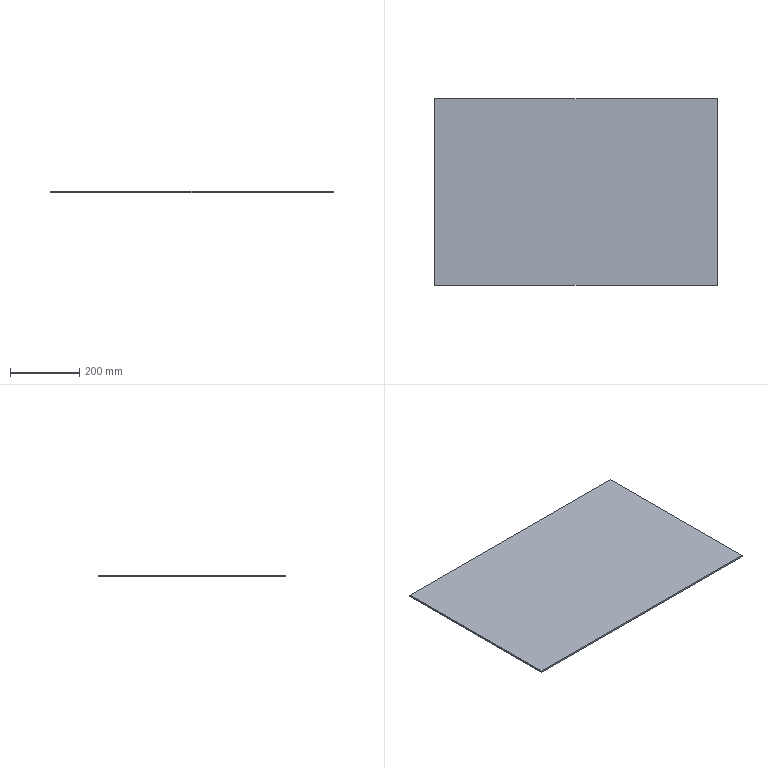Part | STEP file | 1 solid | 10 faces | box 822 x 540 x 5 mm | volume 2219396 mm3 | plane 6 | cylinder 4 | commonest cylinder face diameters 2 x4
STEP:
#1=CARTESIAN_POINT('',(0.,0.,0.));
#2=DIRECTION('',(0.,0.,1.));
#3=DIRECTION('',(1.,0.,0.));
#4=AXIS2_PLACEMENT_3D('',#1,#2,#3);
#5=CARTESIAN_POINT('',(410.,-270.,0.));
#6=VERTEX_POINT('',#5);
#7=CARTESIAN_POINT('',(411.,-269.,0.));
#8=VERTEX_POINT('',#7);
#9=CARTESIAN_POINT('',(410.,-269.,0.));
#10=DIRECTION('',(0.,0.,1.));
#11=DIRECTION('',(-1.,0.,0.));
#12=AXIS2_PLACEMENT_3D('',#9,#10,#11);
#13=CIRCLE('',#12,1.);
#14=CARTESIAN_POINT('',(410.,-269.,5.));
#15=DIRECTION('',(0.,0.,-1.));
#16=DIRECTION('',(-1.,0.,0.));
#17=AXIS2_PLACEMENT_3D('',#14,#15,#16);
#18=CYLINDRICAL_SURFACE('',#17,1.);
#19=CARTESIAN_POINT('',(6.283,5.));
#20=DIRECTION('',(-1.,0.));
#21=VECTOR('',#20,1.);
#22=LINE('',#19,#21);
#23=(GEOMETRIC_REPRESENTATION_CONTEXT(2)PARAMETRIC_REPRESENTATION_CONTEXT()REPRESENTATION_CONTEXT('',''));
#24=DEFINITIONAL_REPRESENTATION('',(#22),#23);
#25=PCURVE('',#18,#24);
#26=CARTESIAN_POINT('',(410.,-269.,0.));
#27=DIRECTION('',(0.,0.,-1.));
#28=DIRECTION('',(-1.,0.,0.));
#29=AXIS2_PLACEMENT_3D('',#26,#27,#28);
#30=PLANE('',#29);
#31=CARTESIAN_POINT('',(1.,0.));
#32=CARTESIAN_POINT('',(1.,-1.732));
#33=CARTESIAN_POINT('',(-0.5,-0.866));
#34=CARTESIAN_POINT('',(-2.,0.));
#35=CARTESIAN_POINT('',(-0.5,0.866));
#36=CARTESIAN_POINT('',(1.,1.732));
#37=CARTESIAN_POINT('',(1.,0.));
#38=(BOUNDED_CURVE()B_SPLINE_CURVE(2,(#31,#32,#33,#34,#35,#36,#37),.UNSPECIFIED.,.T.,.F.)B_SPLINE_CURVE_WITH_KNOTS((1,2,2,2,2,1),(-2.094,0.,2.094,4.189,6.283,8.378),.UNSPECIFIED.)CURVE()GEOMETRIC_REPRESENTATION_ITEM()RATIONAL_B_SPLINE_CURVE((1.,0.5,1.,0.5,1.,0.5,1.))REPRESENTATION_ITEM(''));
#39=(GEOMETRIC_REPRESENTATION_CONTEXT(2)PARAMETRIC_REPRESENTATION_CONTEXT()REPRESENTATION_CONTEXT('',''));
#40=DEFINITIONAL_REPRESENTATION('',(#38),#39);
#41=PCURVE('',#30,#40);
#42=SURFACE_CURVE('',#13,(#25,#41),.PCURVE_S1.);
#43=EDGE_CURVE('',#6,#8,#42,.T.);
#44=ORIENTED_EDGE('',*,*,#43,.T.);
#45=CARTESIAN_POINT('',(411.,-269.,5.));
#46=VERTEX_POINT('',#45);
#47=CARTESIAN_POINT('',(411.,-269.,5.));
#48=DIRECTION('',(0.,0.,-1.));
#49=VECTOR('',#48,1.);
#50=LINE('',#47,#49);
#51=CARTESIAN_POINT('',(3.142,0.));
#52=DIRECTION('',(0.,1.));
#53=VECTOR('',#52,1.);
#54=LINE('',#51,#53);
#55=(GEOMETRIC_REPRESENTATION_CONTEXT(2)PARAMETRIC_REPRESENTATION_CONTEXT()REPRESENTATION_CONTEXT('',''));
#56=DEFINITIONAL_REPRESENTATION('',(#54),#55);
#57=PCURVE('',#18,#56);
#58=CARTESIAN_POINT('',(411.,269.,5.));
#59=DIRECTION('',(-1.,0.,0.));
#60=DIRECTION('',(0.,0.,1.));
#61=AXIS2_PLACEMENT_3D('',#58,#59,#60);
#62=PLANE('',#61);
#63=CARTESIAN_POINT('',(0.,-538.));
#64=DIRECTION('',(-1.,0.));
#65=VECTOR('',#64,1.);
#66=LINE('',#63,#65);
#67=(GEOMETRIC_REPRESENTATION_CONTEXT(2)PARAMETRIC_REPRESENTATION_CONTEXT()REPRESENTATION_CONTEXT('',''));
#68=DEFINITIONAL_REPRESENTATION('',(#66),#67);
#69=PCURVE('',#62,#68);
#70=SURFACE_CURVE('',#50,(#57,#69),.PCURVE_S1.);
#71=EDGE_CURVE('',#46,#8,#70,.T.);
#72=ORIENTED_EDGE('',*,*,#71,.F.);
#73=CARTESIAN_POINT('',(410.,-270.,5.));
#74=VERTEX_POINT('',#73);
#75=CARTESIAN_POINT('',(410.,-269.,5.));
#76=DIRECTION('',(0.,0.,1.));
#77=DIRECTION('',(-1.,0.,0.));
#78=AXIS2_PLACEMENT_3D('',#75,#76,#77);
#79=CIRCLE('',#78,1.);
#80=CARTESIAN_POINT('',(6.283,0.));
#81=DIRECTION('',(-1.,0.));
#82=VECTOR('',#81,1.);
#83=LINE('',#80,#82);
#84=(GEOMETRIC_REPRESENTATION_CONTEXT(2)PARAMETRIC_REPRESENTATION_CONTEXT()REPRESENTATION_CONTEXT('',''));
#85=DEFINITIONAL_REPRESENTATION('',(#83),#84);
#86=PCURVE('',#18,#85);
#87=CARTESIAN_POINT('',(410.,-269.,5.));
#88=DIRECTION('',(0.,0.,-1.));
#89=DIRECTION('',(-1.,0.,0.));
#90=AXIS2_PLACEMENT_3D('',#87,#88,#89);
#91=PLANE('',#90);
#92=CARTESIAN_POINT('',(1.,0.));
#93=CARTESIAN_POINT('',(1.,-1.732));
#94=CARTESIAN_POINT('',(-0.5,-0.866));
#95=CARTESIAN_POINT('',(-2.,0.));
#96=CARTESIAN_POINT('',(-0.5,0.866));
#97=CARTESIAN_POINT('',(1.,1.732));
#98=CARTESIAN_POINT('',(1.,0.));
#99=(BOUNDED_CURVE()B_SPLINE_CURVE(2,(#92,#93,#94,#95,#96,#97,#98),.UNSPECIFIED.,.T.,.F.)B_SPLINE_CURVE_WITH_KNOTS((1,2,2,2,2,1),(-2.094,0.,2.094,4.189,6.283,8.378),.UNSPECIFIED.)CURVE()GEOMETRIC_REPRESENTATION_ITEM()RATIONAL_B_SPLINE_CURVE((1.,0.5,1.,0.5,1.,0.5,1.))REPRESENTATION_ITEM(''));
#100=(GEOMETRIC_REPRESENTATION_CONTEXT(2)PARAMETRIC_REPRESENTATION_CONTEXT()REPRESENTATION_CONTEXT('',''));
#101=DEFINITIONAL_REPRESENTATION('',(#99),#100);
#102=PCURVE('',#91,#101);
#103=SURFACE_CURVE('',#79,(#86,#102),.PCURVE_S1.);
#104=EDGE_CURVE('',#74,#46,#103,.T.);
#105=ORIENTED_EDGE('',*,*,#104,.F.);
#106=CARTESIAN_POINT('',(410.,-270.,5.));
#107=DIRECTION('',(0.,0.,-1.));
#108=VECTOR('',#107,1.);
#109=LINE('',#106,#108);
#110=CARTESIAN_POINT('',(4.712,0.));
#111=DIRECTION('',(0.,1.));
#112=VECTOR('',#111,1.);
#113=LINE('',#110,#112);
#114=(GEOMETRIC_REPRESENTATION_CONTEXT(2)PARAMETRIC_REPRESENTATION_CONTEXT()REPRESENTATION_CONTEXT('',''));
#115=DEFINITIONAL_REPRESENTATION('',(#113),#114);
#116=PCURVE('',#18,#115);
#117=CARTESIAN_POINT('',(-410.,-270.,5.));
#118=DIRECTION('',(0.,1.,0.));
#119=DIRECTION('',(0.,0.,1.));
#120=AXIS2_PLACEMENT_3D('',#117,#118,#119);
#121=PLANE('',#120);
#122=CARTESIAN_POINT('',(0.,820.));
#123=DIRECTION('',(-1.,0.));
#124=VECTOR('',#123,1.);
#125=LINE('',#122,#124);
#126=(GEOMETRIC_REPRESENTATION_CONTEXT(2)PARAMETRIC_REPRESENTATION_CONTEXT()REPRESENTATION_CONTEXT('',''));
#127=DEFINITIONAL_REPRESENTATION('',(#125),#126);
#128=PCURVE('',#121,#127);
#129=SURFACE_CURVE('',#109,(#116,#128),.PCURVE_S1.);
#130=EDGE_CURVE('',#74,#6,#129,.T.);
#131=ORIENTED_EDGE('',*,*,#130,.T.);
#132=EDGE_LOOP('',(#44,#72,#105,#131));
#133=FACE_BOUND('',#132,.T.);
#134=ADVANCED_FACE('',(#133),#18,.T.);
#135=CARTESIAN_POINT('',(411.,269.,0.));
#136=VERTEX_POINT('',#135);
#137=CARTESIAN_POINT('',(411.,269.,0.));
#138=DIRECTION('',(0.,1.,0.));
#139=VECTOR('',#138,1.);
#140=LINE('',#137,#139);
#141=CARTESIAN_POINT('',(-5.,0.));
#142=DIRECTION('',(0.,1.));
#143=VECTOR('',#142,1.);
#144=LINE('',#141,#143);
#145=(GEOMETRIC_REPRESENTATION_CONTEXT(2)PARAMETRIC_REPRESENTATION_CONTEXT()REPRESENTATION_CONTEXT('',''));
#146=DEFINITIONAL_REPRESENTATION('',(#144),#145);
#147=PCURVE('',#62,#146);
#148=CARTESIAN_POINT('',(-1.,538.));
#149=DIRECTION('',(0.,1.));
#150=VECTOR('',#149,1.);
#151=LINE('',#148,#150);
#152=(GEOMETRIC_REPRESENTATION_CONTEXT(2)PARAMETRIC_REPRESENTATION_CONTEXT()REPRESENTATION_CONTEXT('',''));
#153=DEFINITIONAL_REPRESENTATION('',(#151),#152);
#154=PCURVE('',#30,#153);
#155=SURFACE_CURVE('',#140,(#147,#154),.PCURVE_S1.);
#156=EDGE_CURVE('',#8,#136,#155,.T.);
#157=ORIENTED_EDGE('',*,*,#156,.T.);
#158=CARTESIAN_POINT('',(411.,269.,5.));
#159=VERTEX_POINT('',#158);
#160=CARTESIAN_POINT('',(411.,269.,5.));
#161=DIRECTION('',(0.,0.,-1.));
#162=VECTOR('',#161,1.);
#163=LINE('',#160,#162);
#164=CARTESIAN_POINT('',(0.,0.));
#165=DIRECTION('',(-1.,0.));
#166=VECTOR('',#165,1.);
#167=LINE('',#164,#166);
#168=(GEOMETRIC_REPRESENTATION_CONTEXT(2)PARAMETRIC_REPRESENTATION_CONTEXT()REPRESENTATION_CONTEXT('',''));
#169=DEFINITIONAL_REPRESENTATION('',(#167),#168);
#170=PCURVE('',#62,#169);
#171=CARTESIAN_POINT('',(410.,269.,5.));
#172=DIRECTION('',(0.,0.,-1.));
#173=DIRECTION('',(-1.,0.,0.));
#174=AXIS2_PLACEMENT_3D('',#171,#172,#173);
#175=CYLINDRICAL_SURFACE('',#174,1.);
#176=CARTESIAN_POINT('',(3.142,0.));
#177=DIRECTION('',(0.,1.));
#178=VECTOR('',#177,1.);
#179=LINE('',#176,#178);
#180=(GEOMETRIC_REPRESENTATION_CONTEXT(2)PARAMETRIC_REPRESENTATION_CONTEXT()REPRESENTATION_CONTEXT('',''));
#181=DEFINITIONAL_REPRESENTATION('',(#179),#180);
#182=PCURVE('',#175,#181);
#183=SURFACE_CURVE('',#163,(#170,#182),.PCURVE_S1.);
#184=EDGE_CURVE('',#159,#136,#183,.T.);
#185=ORIENTED_EDGE('',*,*,#184,.F.);
#186=CARTESIAN_POINT('',(411.,269.,5.));
#187=DIRECTION('',(0.,1.,0.));
#188=VECTOR('',#187,1.);
#189=LINE('',#186,#188);
#190=CARTESIAN_POINT('',(0.,0.));
#191=DIRECTION('',(0.,1.));
#192=VECTOR('',#191,1.);
#193=LINE('',#190,#192);
#194=(GEOMETRIC_REPRESENTATION_CONTEXT(2)PARAMETRIC_REPRESENTATION_CONTEXT()REPRESENTATION_CONTEXT('',''));
#195=DEFINITIONAL_REPRESENTATION('',(#193),#194);
#196=PCURVE('',#62,#195);
#197=CARTESIAN_POINT('',(-1.,538.));
#198=DIRECTION('',(0.,1.));
#199=VECTOR('',#198,1.);
#200=LINE('',#197,#199);
#201=(GEOMETRIC_REPRESENTATION_CONTEXT(2)PARAMETRIC_REPRESENTATION_CONTEXT()REPRESENTATION_CONTEXT('',''));
#202=DEFINITIONAL_REPRESENTATION('',(#200),#201);
#203=PCURVE('',#91,#202);
#204=SURFACE_CURVE('',#189,(#196,#203),.PCURVE_S1.);
#205=EDGE_CURVE('',#46,#159,#204,.T.);
#206=ORIENTED_EDGE('',*,*,#205,.F.);
#207=ORIENTED_EDGE('',*,*,#71,.T.);
#208=EDGE_LOOP('',(#157,#185,#206,#207));
#209=FACE_BOUND('',#208,.T.);
#210=ADVANCED_FACE('',(#209),#62,.F.);
#211=CARTESIAN_POINT('',(410.,270.,0.));
#212=VERTEX_POINT('',#211);
#213=CARTESIAN_POINT('',(410.,269.,0.));
#214=DIRECTION('',(0.,0.,1.));
#215=DIRECTION('',(1.,0.,0.));
#216=AXIS2_PLACEMENT_3D('',#213,#214,#215);
#217=CIRCLE('',#216,1.);
#218=CARTESIAN_POINT('',(3.142,5.));
#219=DIRECTION('',(-1.,0.));
#220=VECTOR('',#219,1.);
#221=LINE('',#218,#220);
#222=(GEOMETRIC_REPRESENTATION_CONTEXT(2)PARAMETRIC_REPRESENTATION_CONTEXT()REPRESENTATION_CONTEXT('',''));
#223=DEFINITIONAL_REPRESENTATION('',(#221),#222);
#224=PCURVE('',#175,#223);
#225=CARTESIAN_POINT('',(-1.,538.));
#226=CARTESIAN_POINT('',(-1.,539.732));
#227=CARTESIAN_POINT('',(0.5,538.866));
#228=CARTESIAN_POINT('',(2.,538.));
#229=CARTESIAN_POINT('',(0.5,537.134));
#230=CARTESIAN_POINT('',(-1.,536.268));
#231=CARTESIAN_POINT('',(-1.,538.));
#232=(BOUNDED_CURVE()B_SPLINE_CURVE(2,(#225,#226,#227,#228,#229,#230,#231),.UNSPECIFIED.,.T.,.F.)B_SPLINE_CURVE_WITH_KNOTS((1,2,2,2,2,1),(-2.094,0.,2.094,4.189,6.283,8.378),.UNSPECIFIED.)CURVE()GEOMETRIC_REPRESENTATION_ITEM()RATIONAL_B_SPLINE_CURVE((1.,0.5,1.,0.5,1.,0.5,1.))REPRESENTATION_ITEM(''));
#233=(GEOMETRIC_REPRESENTATION_CONTEXT(2)PARAMETRIC_REPRESENTATION_CONTEXT()REPRESENTATION_CONTEXT('',''));
#234=DEFINITIONAL_REPRESENTATION('',(#232),#233);
#235=PCURVE('',#30,#234);
#236=SURFACE_CURVE('',#217,(#224,#235),.PCURVE_S1.);
#237=EDGE_CURVE('',#136,#212,#236,.T.);
#238=ORIENTED_EDGE('',*,*,#237,.T.);
#239=CARTESIAN_POINT('',(410.,270.,5.));
#240=VERTEX_POINT('',#239);
#241=CARTESIAN_POINT('',(410.,270.,5.));
#242=DIRECTION('',(0.,0.,-1.));
#243=VECTOR('',#242,1.);
#244=LINE('',#241,#243);
#245=CARTESIAN_POINT('',(1.571,0.));
#246=DIRECTION('',(0.,1.));
#247=VECTOR('',#246,1.);
#248=LINE('',#245,#247);
#249=(GEOMETRIC_REPRESENTATION_CONTEXT(2)PARAMETRIC_REPRESENTATION_CONTEXT()REPRESENTATION_CONTEXT('',''));
#250=DEFINITIONAL_REPRESENTATION('',(#248),#249);
#251=PCURVE('',#175,#250);
#252=CARTESIAN_POINT('',(-410.,270.,5.));
#253=DIRECTION('',(0.,-1.,0.));
#254=DIRECTION('',(0.,0.,-1.));
#255=AXIS2_PLACEMENT_3D('',#252,#253,#254);
#256=PLANE('',#255);
#257=CARTESIAN_POINT('',(0.,820.));
#258=DIRECTION('',(1.,0.));
#259=VECTOR('',#258,1.);
#260=LINE('',#257,#259);
#261=(GEOMETRIC_REPRESENTATION_CONTEXT(2)PARAMETRIC_REPRESENTATION_CONTEXT()REPRESENTATION_CONTEXT('',''));
#262=DEFINITIONAL_REPRESENTATION('',(#260),#261);
#263=PCURVE('',#256,#262);
#264=SURFACE_CURVE('',#244,(#251,#263),.PCURVE_S1.);
#265=EDGE_CURVE('',#240,#212,#264,.T.);
#266=ORIENTED_EDGE('',*,*,#265,.F.);
#267=CARTESIAN_POINT('',(410.,269.,5.));
#268=DIRECTION('',(0.,0.,1.));
#269=DIRECTION('',(1.,0.,0.));
#270=AXIS2_PLACEMENT_3D('',#267,#268,#269);
#271=CIRCLE('',#270,1.);
#272=CARTESIAN_POINT('',(3.142,0.));
#273=DIRECTION('',(-1.,0.));
#274=VECTOR('',#273,1.);
#275=LINE('',#272,#274);
#276=(GEOMETRIC_REPRESENTATION_CONTEXT(2)PARAMETRIC_REPRESENTATION_CONTEXT()REPRESENTATION_CONTEXT('',''));
#277=DEFINITIONAL_REPRESENTATION('',(#275),#276);
#278=PCURVE('',#175,#277);
#279=CARTESIAN_POINT('',(-1.,538.));
#280=CARTESIAN_POINT('',(-1.,539.732));
#281=CARTESIAN_POINT('',(0.5,538.866));
#282=CARTESIAN_POINT('',(2.,538.));
#283=CARTESIAN_POINT('',(0.5,537.134));
#284=CARTESIAN_POINT('',(-1.,536.268));
#285=CARTESIAN_POINT('',(-1.,538.));
#286=(BOUNDED_CURVE()B_SPLINE_CURVE(2,(#279,#280,#281,#282,#283,#284,#285),.UNSPECIFIED.,.T.,.F.)B_SPLINE_CURVE_WITH_KNOTS((1,2,2,2,2,1),(-2.094,0.,2.094,4.189,6.283,8.378),.UNSPECIFIED.)CURVE()GEOMETRIC_REPRESENTATION_ITEM()RATIONAL_B_SPLINE_CURVE((1.,0.5,1.,0.5,1.,0.5,1.))REPRESENTATION_ITEM(''));
#287=(GEOMETRIC_REPRESENTATION_CONTEXT(2)PARAMETRIC_REPRESENTATION_CONTEXT()REPRESENTATION_CONTEXT('',''));
#288=DEFINITIONAL_REPRESENTATION('',(#286),#287);
#289=PCURVE('',#91,#288);
#290=SURFACE_CURVE('',#271,(#278,#289),.PCURVE_S1.);
#291=EDGE_CURVE('',#159,#240,#290,.T.);
#292=ORIENTED_EDGE('',*,*,#291,.F.);
#293=ORIENTED_EDGE('',*,*,#184,.T.);
#294=EDGE_LOOP('',(#238,#266,#292,#293));
#295=FACE_BOUND('',#294,.T.);
#296=ADVANCED_FACE('',(#295),#175,.T.);
#297=CARTESIAN_POINT('',(-410.,270.,0.));
#298=VERTEX_POINT('',#297);
#299=CARTESIAN_POINT('',(-410.,270.,0.));
#300=DIRECTION('',(-1.,0.,0.));
#301=VECTOR('',#300,1.);
#302=LINE('',#299,#301);
#303=CARTESIAN_POINT('',(5.,0.));
#304=DIRECTION('',(0.,-1.));
#305=VECTOR('',#304,1.);
#306=LINE('',#303,#305);
#307=(GEOMETRIC_REPRESENTATION_CONTEXT(2)PARAMETRIC_REPRESENTATION_CONTEXT()REPRESENTATION_CONTEXT('',''));
#308=DEFINITIONAL_REPRESENTATION('',(#306),#307);
#309=PCURVE('',#256,#308);
#310=CARTESIAN_POINT('',(820.,539.));
#311=DIRECTION('',(1.,0.));
#312=VECTOR('',#311,1.);
#313=LINE('',#310,#312);
#314=(GEOMETRIC_REPRESENTATION_CONTEXT(2)PARAMETRIC_REPRESENTATION_CONTEXT()REPRESENTATION_CONTEXT('',''));
#315=DEFINITIONAL_REPRESENTATION('',(#313),#314);
#316=PCURVE('',#30,#315);
#317=SURFACE_CURVE('',#302,(#309,#316),.PCURVE_S1.);
#318=EDGE_CURVE('',#212,#298,#317,.T.);
#319=ORIENTED_EDGE('',*,*,#318,.T.);
#320=CARTESIAN_POINT('',(-410.,270.,5.));
#321=VERTEX_POINT('',#320);
#322=CARTESIAN_POINT('',(-410.,270.,5.));
#323=DIRECTION('',(0.,0.,-1.));
#324=VECTOR('',#323,1.);
#325=LINE('',#322,#324);
#326=CARTESIAN_POINT('',(0.,0.));
#327=DIRECTION('',(1.,0.));
#328=VECTOR('',#327,1.);
#329=LINE('',#326,#328);
#330=(GEOMETRIC_REPRESENTATION_CONTEXT(2)PARAMETRIC_REPRESENTATION_CONTEXT()REPRESENTATION_CONTEXT('',''));
#331=DEFINITIONAL_REPRESENTATION('',(#329),#330);
#332=PCURVE('',#256,#331);
#333=CARTESIAN_POINT('',(-410.,269.,5.));
#334=DIRECTION('',(0.,0.,-1.));
#335=DIRECTION('',(-1.,0.,0.));
#336=AXIS2_PLACEMENT_3D('',#333,#334,#335);
#337=CYLINDRICAL_SURFACE('',#336,1.);
#338=CARTESIAN_POINT('',(1.571,0.));
#339=DIRECTION('',(0.,1.));
#340=VECTOR('',#339,1.);
#341=LINE('',#338,#340);
#342=(GEOMETRIC_REPRESENTATION_CONTEXT(2)PARAMETRIC_REPRESENTATION_CONTEXT()REPRESENTATION_CONTEXT('',''));
#343=DEFINITIONAL_REPRESENTATION('',(#341),#342);
#344=PCURVE('',#337,#343);
#345=SURFACE_CURVE('',#325,(#332,#344),.PCURVE_S1.);
#346=EDGE_CURVE('',#321,#298,#345,.T.);
#347=ORIENTED_EDGE('',*,*,#346,.F.);
#348=CARTESIAN_POINT('',(-410.,270.,5.));
#349=DIRECTION('',(-1.,0.,0.));
#350=VECTOR('',#349,1.);
#351=LINE('',#348,#350);
#352=CARTESIAN_POINT('',(0.,0.));
#353=DIRECTION('',(0.,-1.));
#354=VECTOR('',#353,1.);
#355=LINE('',#352,#354);
#356=(GEOMETRIC_REPRESENTATION_CONTEXT(2)PARAMETRIC_REPRESENTATION_CONTEXT()REPRESENTATION_CONTEXT('',''));
#357=DEFINITIONAL_REPRESENTATION('',(#355),#356);
#358=PCURVE('',#256,#357);
#359=CARTESIAN_POINT('',(820.,539.));
#360=DIRECTION('',(1.,0.));
#361=VECTOR('',#360,1.);
#362=LINE('',#359,#361);
#363=(GEOMETRIC_REPRESENTATION_CONTEXT(2)PARAMETRIC_REPRESENTATION_CONTEXT()REPRESENTATION_CONTEXT('',''));
#364=DEFINITIONAL_REPRESENTATION('',(#362),#363);
#365=PCURVE('',#91,#364);
#366=SURFACE_CURVE('',#351,(#358,#365),.PCURVE_S1.);
#367=EDGE_CURVE('',#240,#321,#366,.T.);
#368=ORIENTED_EDGE('',*,*,#367,.F.);
#369=ORIENTED_EDGE('',*,*,#265,.T.);
#370=EDGE_LOOP('',(#319,#347,#368,#369));
#371=FACE_BOUND('',#370,.T.);
#372=ADVANCED_FACE('',(#371),#256,.F.);
#373=CARTESIAN_POINT('',(-411.,269.,0.));
#374=VERTEX_POINT('',#373);
#375=CARTESIAN_POINT('',(-410.,269.,0.));
#376=DIRECTION('',(0.,0.,1.));
#377=DIRECTION('',(-1.,0.,0.));
#378=AXIS2_PLACEMENT_3D('',#375,#376,#377);
#379=CIRCLE('',#378,1.);
#380=CARTESIAN_POINT('',(6.283,5.));
#381=DIRECTION('',(-1.,0.));
#382=VECTOR('',#381,1.);
#383=LINE('',#380,#382);
#384=(GEOMETRIC_REPRESENTATION_CONTEXT(2)PARAMETRIC_REPRESENTATION_CONTEXT()REPRESENTATION_CONTEXT('',''));
#385=DEFINITIONAL_REPRESENTATION('',(#383),#384);
#386=PCURVE('',#337,#385);
#387=CARTESIAN_POINT('',(821.,538.));
#388=CARTESIAN_POINT('',(821.,536.268));
#389=CARTESIAN_POINT('',(819.5,537.134));
#390=CARTESIAN_POINT('',(818.,538.));
#391=CARTESIAN_POINT('',(819.5,538.866));
#392=CARTESIAN_POINT('',(821.,539.732));
#393=CARTESIAN_POINT('',(821.,538.));
#394=(BOUNDED_CURVE()B_SPLINE_CURVE(2,(#387,#388,#389,#390,#391,#392,#393),.UNSPECIFIED.,.T.,.F.)B_SPLINE_CURVE_WITH_KNOTS((1,2,2,2,2,1),(-2.094,0.,2.094,4.189,6.283,8.378),.UNSPECIFIED.)CURVE()GEOMETRIC_REPRESENTATION_ITEM()RATIONAL_B_SPLINE_CURVE((1.,0.5,1.,0.5,1.,0.5,1.))REPRESENTATION_ITEM(''));
#395=(GEOMETRIC_REPRESENTATION_CONTEXT(2)PARAMETRIC_REPRESENTATION_CONTEXT()REPRESENTATION_CONTEXT('',''));
#396=DEFINITIONAL_REPRESENTATION('',(#394),#395);
#397=PCURVE('',#30,#396);
#398=SURFACE_CURVE('',#379,(#386,#397),.PCURVE_S1.);
#399=EDGE_CURVE('',#298,#374,#398,.T.);
#400=ORIENTED_EDGE('',*,*,#399,.T.);
#401=CARTESIAN_POINT('',(-411.,269.,5.));
#402=VERTEX_POINT('',#401);
#403=CARTESIAN_POINT('',(-411.,269.,5.));
#404=DIRECTION('',(0.,0.,-1.));
#405=VECTOR('',#404,1.);
#406=LINE('',#403,#405);
#407=CARTESIAN_POINT('',(0.,0.));
#408=DIRECTION('',(0.,1.));
#409=VECTOR('',#408,1.);
#410=LINE('',#407,#409);
#411=(GEOMETRIC_REPRESENTATION_CONTEXT(2)PARAMETRIC_REPRESENTATION_CONTEXT()REPRESENTATION_CONTEXT('',''));
#412=DEFINITIONAL_REPRESENTATION('',(#410),#411);
#413=PCURVE('',#337,#412);
#414=CARTESIAN_POINT('',(-411.,269.,5.));
#415=DIRECTION('',(1.,0.,0.));
#416=DIRECTION('',(0.,1.,0.));
#417=AXIS2_PLACEMENT_3D('',#414,#415,#416);
#418=PLANE('',#417);
#419=CARTESIAN_POINT('',(0.,0.));
#420=DIRECTION('',(0.,-1.));
#421=VECTOR('',#420,1.);
#422=LINE('',#419,#421);
#423=(GEOMETRIC_REPRESENTATION_CONTEXT(2)PARAMETRIC_REPRESENTATION_CONTEXT()REPRESENTATION_CONTEXT('',''));
#424=DEFINITIONAL_REPRESENTATION('',(#422),#423);
#425=PCURVE('',#418,#424);
#426=SURFACE_CURVE('',#406,(#413,#425),.PCURVE_S1.);
#427=EDGE_CURVE('',#402,#374,#426,.T.);
#428=ORIENTED_EDGE('',*,*,#427,.F.);
#429=CARTESIAN_POINT('',(-410.,269.,5.));
#430=DIRECTION('',(0.,0.,1.));
#431=DIRECTION('',(-1.,0.,0.));
#432=AXIS2_PLACEMENT_3D('',#429,#430,#431);
#433=CIRCLE('',#432,1.);
#434=CARTESIAN_POINT('',(6.283,0.));
#435=DIRECTION('',(-1.,0.));
#436=VECTOR('',#435,1.);
#437=LINE('',#434,#436);
#438=(GEOMETRIC_REPRESENTATION_CONTEXT(2)PARAMETRIC_REPRESENTATION_CONTEXT()REPRESENTATION_CONTEXT('',''));
#439=DEFINITIONAL_REPRESENTATION('',(#437),#438);
#440=PCURVE('',#337,#439);
#441=CARTESIAN_POINT('',(821.,538.));
#442=CARTESIAN_POINT('',(821.,536.268));
#443=CARTESIAN_POINT('',(819.5,537.134));
#444=CARTESIAN_POINT('',(818.,538.));
#445=CARTESIAN_POINT('',(819.5,538.866));
#446=CARTESIAN_POINT('',(821.,539.732));
#447=CARTESIAN_POINT('',(821.,538.));
#448=(BOUNDED_CURVE()B_SPLINE_CURVE(2,(#441,#442,#443,#444,#445,#446,#447),.UNSPECIFIED.,.T.,.F.)B_SPLINE_CURVE_WITH_KNOTS((1,2,2,2,2,1),(-2.094,0.,2.094,4.189,6.283,8.378),.UNSPECIFIED.)CURVE()GEOMETRIC_REPRESENTATION_ITEM()RATIONAL_B_SPLINE_CURVE((1.,0.5,1.,0.5,1.,0.5,1.))REPRESENTATION_ITEM(''));
#449=(GEOMETRIC_REPRESENTATION_CONTEXT(2)PARAMETRIC_REPRESENTATION_CONTEXT()REPRESENTATION_CONTEXT('',''));
#450=DEFINITIONAL_REPRESENTATION('',(#448),#449);
#451=PCURVE('',#91,#450);
#452=SURFACE_CURVE('',#433,(#440,#451),.PCURVE_S1.);
#453=EDGE_CURVE('',#321,#402,#452,.T.);
#454=ORIENTED_EDGE('',*,*,#453,.F.);
#455=ORIENTED_EDGE('',*,*,#346,.T.);
#456=EDGE_LOOP('',(#400,#428,#454,#455));
#457=FACE_BOUND('',#456,.T.);
#458=ADVANCED_FACE('',(#457),#337,.T.);
#459=CARTESIAN_POINT('',(-411.,-269.,0.));
#460=VERTEX_POINT('',#459);
#461=CARTESIAN_POINT('',(-411.,269.,0.));
#462=DIRECTION('',(0.,-1.,0.));
#463=VECTOR('',#462,1.);
#464=LINE('',#461,#463);
#465=CARTESIAN_POINT('',(0.,-5.));
#466=DIRECTION('',(-1.,0.));
#467=VECTOR('',#466,1.);
#468=LINE('',#465,#467);
#469=(GEOMETRIC_REPRESENTATION_CONTEXT(2)PARAMETRIC_REPRESENTATION_CONTEXT()REPRESENTATION_CONTEXT('',''));
#470=DEFINITIONAL_REPRESENTATION('',(#468),#469);
#471=PCURVE('',#418,#470);
#472=CARTESIAN_POINT('',(821.,538.));
#473=DIRECTION('',(0.,-1.));
#474=VECTOR('',#473,1.);
#475=LINE('',#472,#474);
#476=(GEOMETRIC_REPRESENTATION_CONTEXT(2)PARAMETRIC_REPRESENTATION_CONTEXT()REPRESENTATION_CONTEXT('',''));
#477=DEFINITIONAL_REPRESENTATION('',(#475),#476);
#478=PCURVE('',#30,#477);
#479=SURFACE_CURVE('',#464,(#471,#478),.PCURVE_S1.);
#480=EDGE_CURVE('',#374,#460,#479,.T.);
#481=ORIENTED_EDGE('',*,*,#480,.T.);
#482=CARTESIAN_POINT('',(-411.,-269.,5.));
#483=VERTEX_POINT('',#482);
#484=CARTESIAN_POINT('',(-411.,-269.,5.));
#485=DIRECTION('',(0.,0.,-1.));
#486=VECTOR('',#485,1.);
#487=LINE('',#484,#486);
#488=CARTESIAN_POINT('',(-538.,0.));
#489=DIRECTION('',(0.,-1.));
#490=VECTOR('',#489,1.);
#491=LINE('',#488,#490);
#492=(GEOMETRIC_REPRESENTATION_CONTEXT(2)PARAMETRIC_REPRESENTATION_CONTEXT()REPRESENTATION_CONTEXT('',''));
#493=DEFINITIONAL_REPRESENTATION('',(#491),#492);
#494=PCURVE('',#418,#493);
#495=CARTESIAN_POINT('',(-410.,-269.,5.));
#496=DIRECTION('',(0.,0.,-1.));
#497=DIRECTION('',(-1.,0.,0.));
#498=AXIS2_PLACEMENT_3D('',#495,#496,#497);
#499=CYLINDRICAL_SURFACE('',#498,1.);
#500=CARTESIAN_POINT('',(6.283,0.));
#501=DIRECTION('',(0.,1.));
#502=VECTOR('',#501,1.);
#503=LINE('',#500,#502);
#504=(GEOMETRIC_REPRESENTATION_CONTEXT(2)PARAMETRIC_REPRESENTATION_CONTEXT()REPRESENTATION_CONTEXT('',''));
#505=DEFINITIONAL_REPRESENTATION('',(#503),#504);
#506=PCURVE('',#499,#505);
#507=SURFACE_CURVE('',#487,(#494,#506),.PCURVE_S1.);
#508=EDGE_CURVE('',#483,#460,#507,.T.);
#509=ORIENTED_EDGE('',*,*,#508,.F.);
#510=CARTESIAN_POINT('',(-411.,269.,5.));
#511=DIRECTION('',(0.,-1.,0.));
#512=VECTOR('',#511,1.);
#513=LINE('',#510,#512);
#514=CARTESIAN_POINT('',(0.,0.));
#515=DIRECTION('',(-1.,0.));
#516=VECTOR('',#515,1.);
#517=LINE('',#514,#516);
#518=(GEOMETRIC_REPRESENTATION_CONTEXT(2)PARAMETRIC_REPRESENTATION_CONTEXT()REPRESENTATION_CONTEXT('',''));
#519=DEFINITIONAL_REPRESENTATION('',(#517),#518);
#520=PCURVE('',#418,#519);
#521=CARTESIAN_POINT('',(821.,538.));
#522=DIRECTION('',(0.,-1.));
#523=VECTOR('',#522,1.);
#524=LINE('',#521,#523);
#525=(GEOMETRIC_REPRESENTATION_CONTEXT(2)PARAMETRIC_REPRESENTATION_CONTEXT()REPRESENTATION_CONTEXT('',''));
#526=DEFINITIONAL_REPRESENTATION('',(#524),#525);
#527=PCURVE('',#91,#526);
#528=SURFACE_CURVE('',#513,(#520,#527),.PCURVE_S1.);
#529=EDGE_CURVE('',#402,#483,#528,.T.);
#530=ORIENTED_EDGE('',*,*,#529,.F.);
#531=ORIENTED_EDGE('',*,*,#427,.T.);
#532=EDGE_LOOP('',(#481,#509,#530,#531));
#533=FACE_BOUND('',#532,.T.);
#534=ADVANCED_FACE('',(#533),#418,.F.);
#535=CARTESIAN_POINT('',(-410.,-270.,0.));
#536=VERTEX_POINT('',#535);
#537=CARTESIAN_POINT('',(-410.,-269.,0.));
#538=DIRECTION('',(0.,0.,1.));
#539=DIRECTION('',(-1.,0.,0.));
#540=AXIS2_PLACEMENT_3D('',#537,#538,#539);
#541=CIRCLE('',#540,1.);
#542=CARTESIAN_POINT('',(6.283,5.));
#543=DIRECTION('',(-1.,0.));
#544=VECTOR('',#543,1.);
#545=LINE('',#542,#544);
#546=(GEOMETRIC_REPRESENTATION_CONTEXT(2)PARAMETRIC_REPRESENTATION_CONTEXT()REPRESENTATION_CONTEXT('',''));
#547=DEFINITIONAL_REPRESENTATION('',(#545),#546);
#548=PCURVE('',#499,#547);
#549=CARTESIAN_POINT('',(821.,0.));
#550=CARTESIAN_POINT('',(821.,-1.732));
#551=CARTESIAN_POINT('',(819.5,-0.866));
#552=CARTESIAN_POINT('',(818.,0.));
#553=CARTESIAN_POINT('',(819.5,0.866));
#554=CARTESIAN_POINT('',(821.,1.732));
#555=CARTESIAN_POINT('',(821.,0.));
#556=(BOUNDED_CURVE()B_SPLINE_CURVE(2,(#549,#550,#551,#552,#553,#554,#555),.UNSPECIFIED.,.T.,.F.)B_SPLINE_CURVE_WITH_KNOTS((1,2,2,2,2,1),(-2.094,0.,2.094,4.189,6.283,8.378),.UNSPECIFIED.)CURVE()GEOMETRIC_REPRESENTATION_ITEM()RATIONAL_B_SPLINE_CURVE((1.,0.5,1.,0.5,1.,0.5,1.))REPRESENTATION_ITEM(''));
#557=(GEOMETRIC_REPRESENTATION_CONTEXT(2)PARAMETRIC_REPRESENTATION_CONTEXT()REPRESENTATION_CONTEXT('',''));
#558=DEFINITIONAL_REPRESENTATION('',(#556),#557);
#559=PCURVE('',#30,#558);
#560=SURFACE_CURVE('',#541,(#548,#559),.PCURVE_S1.);
#561=EDGE_CURVE('',#460,#536,#560,.T.);
#562=ORIENTED_EDGE('',*,*,#561,.T.);
#563=CARTESIAN_POINT('',(-410.,-270.,5.));
#564=VERTEX_POINT('',#563);
#565=CARTESIAN_POINT('',(-410.,-270.,5.));
#566=DIRECTION('',(0.,0.,-1.));
#567=VECTOR('',#566,1.);
#568=LINE('',#565,#567);
#569=CARTESIAN_POINT('',(4.712,0.));
#570=DIRECTION('',(0.,1.));
#571=VECTOR('',#570,1.);
#572=LINE('',#569,#571);
#573=(GEOMETRIC_REPRESENTATION_CONTEXT(2)PARAMETRIC_REPRESENTATION_CONTEXT()REPRESENTATION_CONTEXT('',''));
#574=DEFINITIONAL_REPRESENTATION('',(#572),#573);
#575=PCURVE('',#499,#574);
#576=CARTESIAN_POINT('',(0.,0.));
#577=DIRECTION('',(-1.,0.));
#578=VECTOR('',#577,1.);
#579=LINE('',#576,#578);
#580=(GEOMETRIC_REPRESENTATION_CONTEXT(2)PARAMETRIC_REPRESENTATION_CONTEXT()REPRESENTATION_CONTEXT('',''));
#581=DEFINITIONAL_REPRESENTATION('',(#579),#580);
#582=PCURVE('',#121,#581);
#583=SURFACE_CURVE('',#568,(#575,#582),.PCURVE_S1.);
#584=EDGE_CURVE('',#564,#536,#583,.T.);
#585=ORIENTED_EDGE('',*,*,#584,.F.);
#586=CARTESIAN_POINT('',(-410.,-269.,5.));
#587=DIRECTION('',(0.,0.,1.));
#588=DIRECTION('',(-1.,0.,0.));
#589=AXIS2_PLACEMENT_3D('',#586,#587,#588);
#590=CIRCLE('',#589,1.);
#591=CARTESIAN_POINT('',(6.283,0.));
#592=DIRECTION('',(-1.,0.));
#593=VECTOR('',#592,1.);
#594=LINE('',#591,#593);
#595=(GEOMETRIC_REPRESENTATION_CONTEXT(2)PARAMETRIC_REPRESENTATION_CONTEXT()REPRESENTATION_CONTEXT('',''));
#596=DEFINITIONAL_REPRESENTATION('',(#594),#595);
#597=PCURVE('',#499,#596);
#598=CARTESIAN_POINT('',(821.,0.));
#599=CARTESIAN_POINT('',(821.,-1.732));
#600=CARTESIAN_POINT('',(819.5,-0.866));
#601=CARTESIAN_POINT('',(818.,0.));
#602=CARTESIAN_POINT('',(819.5,0.866));
#603=CARTESIAN_POINT('',(821.,1.732));
#604=CARTESIAN_POINT('',(821.,0.));
#605=(BOUNDED_CURVE()B_SPLINE_CURVE(2,(#598,#599,#600,#601,#602,#603,#604),.UNSPECIFIED.,.T.,.F.)B_SPLINE_CURVE_WITH_KNOTS((1,2,2,2,2,1),(-2.094,0.,2.094,4.189,6.283,8.378),.UNSPECIFIED.)CURVE()GEOMETRIC_REPRESENTATION_ITEM()RATIONAL_B_SPLINE_CURVE((1.,0.5,1.,0.5,1.,0.5,1.))REPRESENTATION_ITEM(''));
#606=(GEOMETRIC_REPRESENTATION_CONTEXT(2)PARAMETRIC_REPRESENTATION_CONTEXT()REPRESENTATION_CONTEXT('',''));
#607=DEFINITIONAL_REPRESENTATION('',(#605),#606);
#608=PCURVE('',#91,#607);
#609=SURFACE_CURVE('',#590,(#597,#608),.PCURVE_S1.);
#610=EDGE_CURVE('',#483,#564,#609,.T.);
#611=ORIENTED_EDGE('',*,*,#610,.F.);
#612=ORIENTED_EDGE('',*,*,#508,.T.);
#613=EDGE_LOOP('',(#562,#585,#611,#612));
#614=FACE_BOUND('',#613,.T.);
#615=ADVANCED_FACE('',(#614),#499,.T.);
#616=CARTESIAN_POINT('',(-410.,-270.,0.));
#617=DIRECTION('',(1.,0.,0.));
#618=VECTOR('',#617,1.);
#619=LINE('',#616,#618);
#620=CARTESIAN_POINT('',(-5.,0.));
#621=DIRECTION('',(0.,1.));
#622=VECTOR('',#621,1.);
#623=LINE('',#620,#622);
#624=(GEOMETRIC_REPRESENTATION_CONTEXT(2)PARAMETRIC_REPRESENTATION_CONTEXT()REPRESENTATION_CONTEXT('',''));
#625=DEFINITIONAL_REPRESENTATION('',(#623),#624);
#626=PCURVE('',#121,#625);
#627=CARTESIAN_POINT('',(820.,-1.));
#628=DIRECTION('',(-1.,0.));
#629=VECTOR('',#628,1.);
#630=LINE('',#627,#629);
#631=(GEOMETRIC_REPRESENTATION_CONTEXT(2)PARAMETRIC_REPRESENTATION_CONTEXT()REPRESENTATION_CONTEXT('',''));
#632=DEFINITIONAL_REPRESENTATION('',(#630),#631);
#633=PCURVE('',#30,#632);
#634=SURFACE_CURVE('',#619,(#626,#633),.PCURVE_S1.);
#635=EDGE_CURVE('',#536,#6,#634,.T.);
#636=ORIENTED_EDGE('',*,*,#635,.T.);
#637=ORIENTED_EDGE('',*,*,#130,.F.);
#638=CARTESIAN_POINT('',(-410.,-270.,5.));
#639=DIRECTION('',(1.,0.,0.));
#640=VECTOR('',#639,1.);
#641=LINE('',#638,#640);
#642=CARTESIAN_POINT('',(0.,0.));
#643=DIRECTION('',(0.,1.));
#644=VECTOR('',#643,1.);
#645=LINE('',#642,#644);
#646=(GEOMETRIC_REPRESENTATION_CONTEXT(2)PARAMETRIC_REPRESENTATION_CONTEXT()REPRESENTATION_CONTEXT('',''));
#647=DEFINITIONAL_REPRESENTATION('',(#645),#646);
#648=PCURVE('',#121,#647);
#649=CARTESIAN_POINT('',(820.,-1.));
#650=DIRECTION('',(-1.,0.));
#651=VECTOR('',#650,1.);
#652=LINE('',#649,#651);
#653=(GEOMETRIC_REPRESENTATION_CONTEXT(2)PARAMETRIC_REPRESENTATION_CONTEXT()REPRESENTATION_CONTEXT('',''));
#654=DEFINITIONAL_REPRESENTATION('',(#652),#653);
#655=PCURVE('',#91,#654);
#656=SURFACE_CURVE('',#641,(#648,#655),.PCURVE_S1.);
#657=EDGE_CURVE('',#564,#74,#656,.T.);
#658=ORIENTED_EDGE('',*,*,#657,.F.);
#659=ORIENTED_EDGE('',*,*,#584,.T.);
#660=EDGE_LOOP('',(#636,#637,#658,#659));
#661=FACE_BOUND('',#660,.T.);
#662=ADVANCED_FACE('',(#661),#121,.F.);
#663=ORIENTED_EDGE('',*,*,#104,.T.);
#664=ORIENTED_EDGE('',*,*,#205,.T.);
#665=ORIENTED_EDGE('',*,*,#291,.T.);
#666=ORIENTED_EDGE('',*,*,#367,.T.);
#667=ORIENTED_EDGE('',*,*,#453,.T.);
#668=ORIENTED_EDGE('',*,*,#529,.T.);
#669=ORIENTED_EDGE('',*,*,#610,.T.);
#670=ORIENTED_EDGE('',*,*,#657,.T.);
#671=EDGE_LOOP('',(#663,#664,#665,#666,#667,#668,#669,#670));
#672=FACE_BOUND('',#671,.T.);
#673=ADVANCED_FACE('',(#672),#91,.F.);
#674=ORIENTED_EDGE('',*,*,#43,.F.);
#675=ORIENTED_EDGE('',*,*,#635,.F.);
#676=ORIENTED_EDGE('',*,*,#561,.F.);
#677=ORIENTED_EDGE('',*,*,#480,.F.);
#678=ORIENTED_EDGE('',*,*,#399,.F.);
#679=ORIENTED_EDGE('',*,*,#318,.F.);
#680=ORIENTED_EDGE('',*,*,#237,.F.);
#681=ORIENTED_EDGE('',*,*,#156,.F.);
#682=EDGE_LOOP('',(#674,#675,#676,#677,#678,#679,#680,#681));
#683=FACE_BOUND('',#682,.T.);
#684=ADVANCED_FACE('',(#683),#30,.T.);
#685=CLOSED_SHELL('',(#134,#210,#296,#372,#458,#534,#615,#662,#673,#684));
#686=MANIFOLD_SOLID_BREP('',#685);
#687=(LENGTH_UNIT()NAMED_UNIT(*)SI_UNIT(.MILLI.,.METRE.));
#688=UNCERTAINTY_MEASURE_WITH_UNIT(LENGTH_MEASURE(0.0000001),#687,'','');
#689=(NAMED_UNIT(*)PLANE_ANGLE_UNIT()SI_UNIT($,.RADIAN.));
#690=(NAMED_UNIT(*)SI_UNIT($,.STERADIAN.)SOLID_ANGLE_UNIT());
#691=(GEOMETRIC_REPRESENTATION_CONTEXT(3)GLOBAL_UNCERTAINTY_ASSIGNED_CONTEXT((#688))GLOBAL_UNIT_ASSIGNED_CONTEXT((#687,#689,#690))REPRESENTATION_CONTEXT('',''));
#692=ADVANCED_BREP_SHAPE_REPRESENTATION('',(#4,#686),#691);